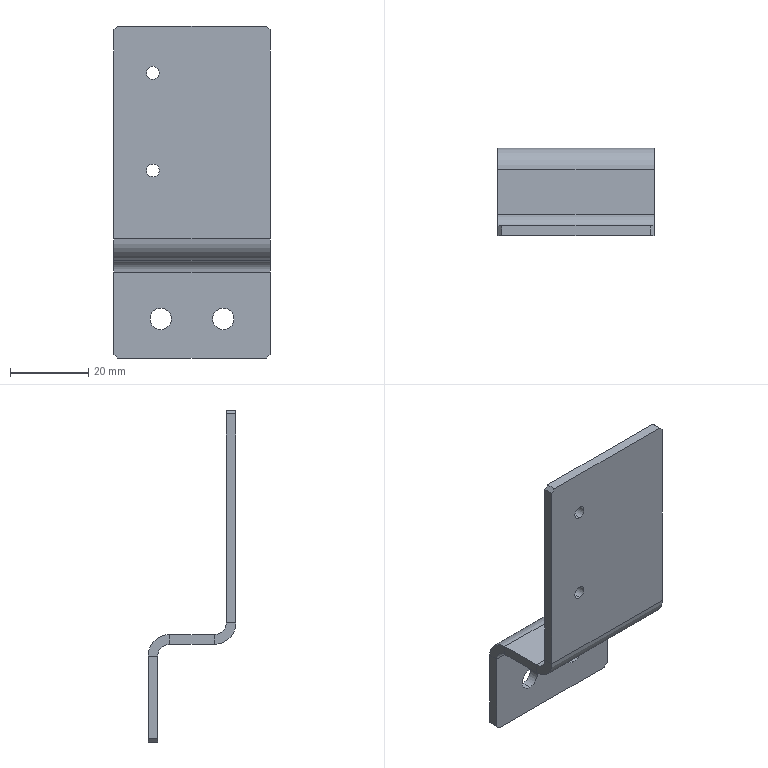Part | STEP file | 227h056253 BKT_Default | 1 solid | 34 faces | box 40 x 22.5 x 85 mm | volume 9969 mm3 | plane 22 | cylinder 12 | commonest cylinder face diameters 3.3 x4 5.5 x4 6 x2 11 x2